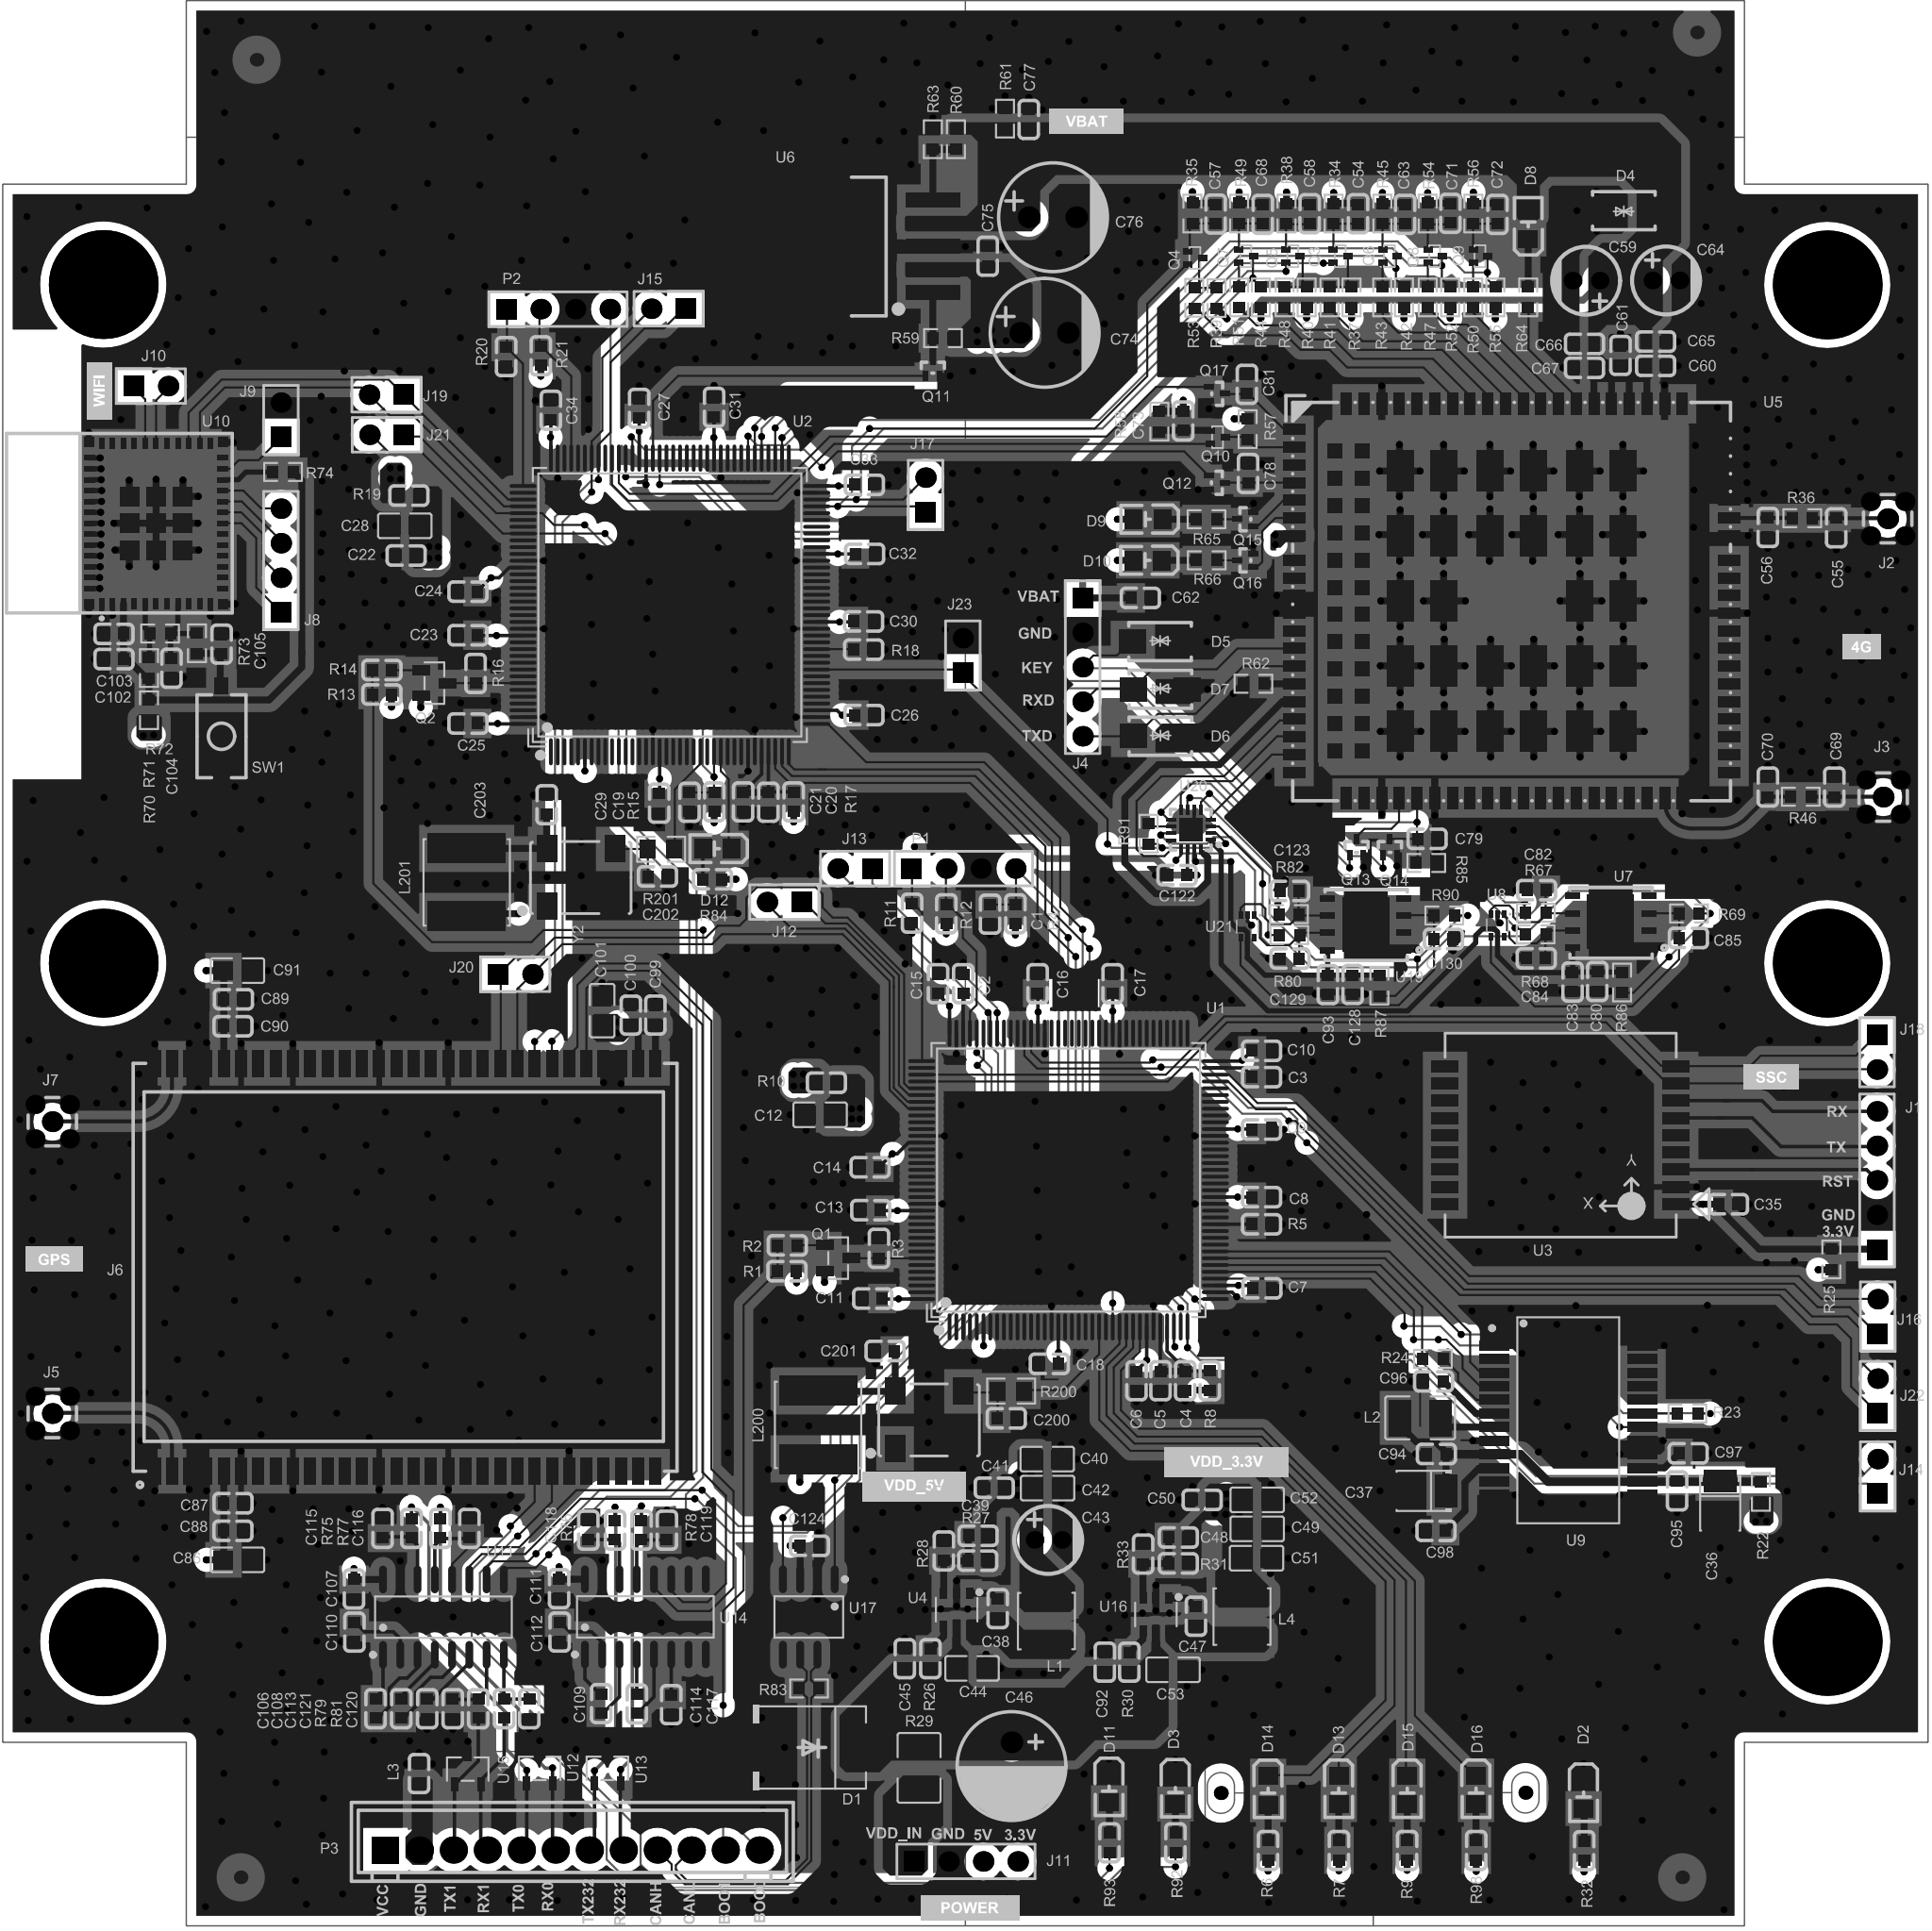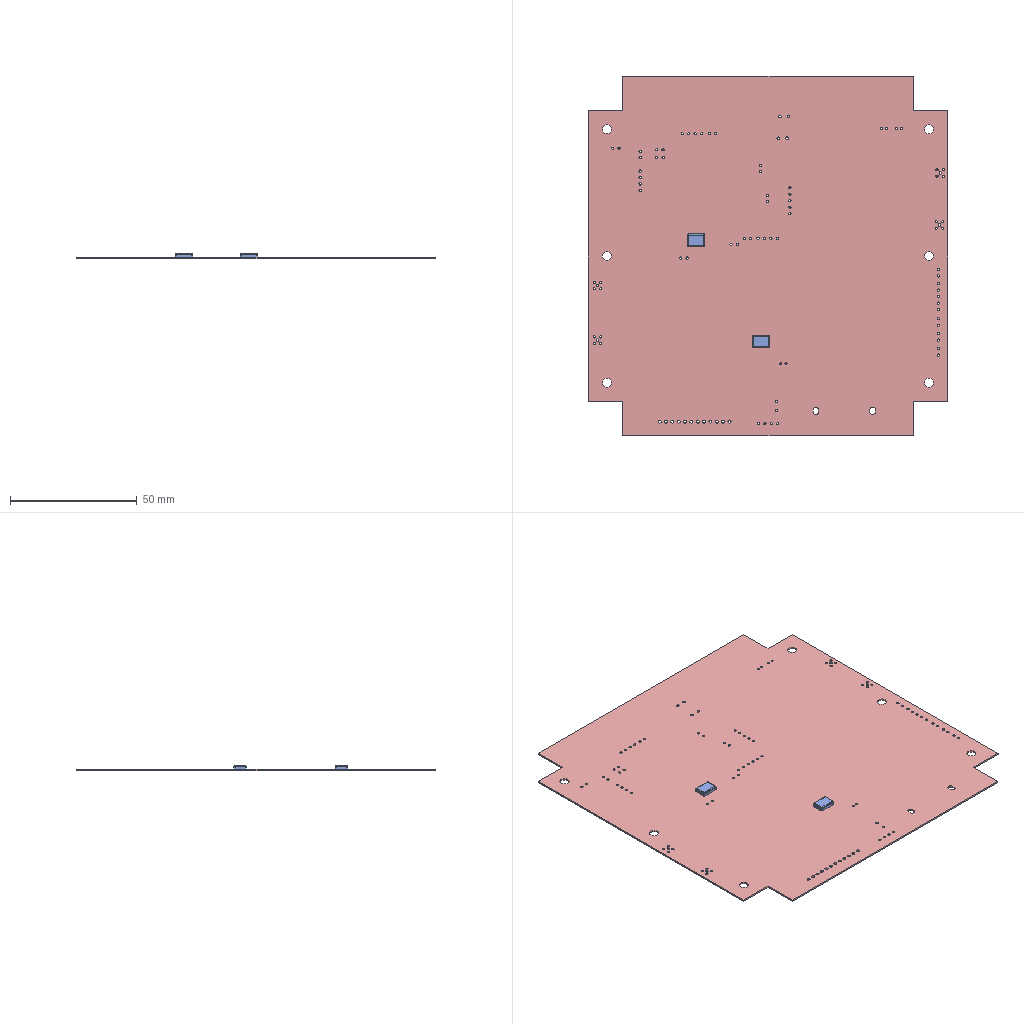Circuit board layout | Altium Designer | box 141.6 x 141.6 x 2.1 mm
Layer stack:
# Altium Designer layer stack of  (unit mm; dielectric type: 0 none, 1 core, 2 prepreg, 3 surface material)
index,name,kind,layer,copper_thickness_mm,dielectric_type,dielectric_thickness_mm,dielectric_material,dielectric_constant
0,Top Paste,other,,,,,,
1,Top Overlay,other,,,,,,
2,Top Solder,dielectric,,,3,0.0102,Solder Resist,3.5
3,Top,copper,Top,0.0356,,,,
4,Dielectric1,dielectric,,,2,0.0711,PP-006,4.1
5,GND02,copper,GND02,0.035,,,,
6,Dielectric5,dielectric,,,0,0.32,FR-4,4.8
7,PWR03,copper,PWR03,0.035,,,,
8,Dielectric6,dielectric,,,2,0.0711,PP-006,4.1
9,Bottom,copper,Bottom,0.0356,,,,
10,Bottom Solder,dielectric,,,3,0.0102,Solder Resist,3.5
11,Bottom Overlay,other,,,,,,
12,Bottom Paste,other,,,,,,
# drill layer pairs: low layer,high layer
drill_pair,Top,Bottom
Part placement:
Designator,Comment,Layer,Footprint,Center-X(mm),Center-Y(mm),Rotation
J11,Single-row straight pin header,TopLayer,HDR1X4,234.391,4.724,360
R85,10K,TopLayer,R0603,268.25,78.159,360
R84,NA,TopLayer,0603,215.74,76.965,180
J23,Boot Option-2.54-single-row pin header,TopLayer,HDR_1X2_254,234.163,93.421,90
J22,Boot Option-2.54-single-row pin header,TopLayer,HDR_1X2_254,301.447,38.964,90
J21,Boot Option-2.54-single-row pin header,TopLayer,HDR_1X2_254,191.795,109.652,180
J20,Boot Option-2.54-single-row pin header,TopLayer,HDR_1X2_254,201.244,69.977,360
J19,Boot Option-2.54-single-row pin header,TopLayer,HDR_1X2_254,191.77,112.598,180
J18,Boot Option-2.54-single-row pin header,TopLayer,HDR_1X2_254,301.396,64.237,270
J17,Boot Option-2.54-single-row pin header,TopLayer,HDR_1X2_254,231.419,105.232,90
J16,Boot Option-2.54-single-row pin header,TopLayer,HDR_1X2_254,301.447,44.806,90
J15,Boot Option-2.54-single-row pin header,TopLayer,HDR_1X2_254,212.522,118.923,180
J14,Boot Option-2.54-single-row pin header,TopLayer,HDR_1X2_254,301.447,33.045,90
J13,Boot Option-2.54-single-row pin header,TopLayer,HDR_1X2_254,226.238,77.749,180
D12,RED,TopLayer,LED_0805,216.089,79.209,360
C96,470nF/50V,TopLayer,0603,268.775,40.033,180
U21,ESDA6V8V6-6,TopLayer,SOT-563,255.092,73.482,90
U16,SY8113B,TopLayer,TSOT-23-6_L2.9-W1.6-P0.95-LS2.8-BR,248.361,22.885,90
U4,SY8113B,TopLayer,TSOT-23-6_L2.9-W1.6-P0.95-LS2.8-BR,233.705,23.241,90
R90,22R,TopLayer,R0603,269.571,74.297,180
R82,22R,TopLayer,R0603,258.149,74.397,360
R80,22R,TopLayer,R0603,258.174,72.859,360
R33,22.1K,TopLayer,0603,247.419,27.323,270
R32,1K,TopLayer,0603,279.854,5.504,270
R31,100K,TopLayer,0603,250.02,26.642,360
R30,100K,TopLayer,0603,246.403,19.372,270
R29,12V/2A,TopLayer,1210,230.944,11.607,270
R28,10K,TopLayer,0603,232.763,27.551,270
R27,75K 1%,TopLayer,0603,235.262,26.845,360
R26,100K,TopLayer,0603,231.772,19.627,270
R25,0R,TopLayer,R0603,298.04,48.997,90
R24,0R,TopLayer,R0603,268.733,41.685,360
R23,0R,TopLayer,R0603,287.451,37.665,180
R22,0R,TopLayer,R0603,292.859,31.903,90
L1,2.2uH/2A,TopLayer,IND-SMD_L4.0-W4.0,240.309,22.403,90
D11,RED,TopLayer,LED_0805,244.921,10.095,90
D3,RED,TopLayer,LED_0805,249.798,9.994,90
D2,RED,TopLayer,LED_0805,279.82,9.663,90
D1,SMCJ18A,TopLayer,SMC_L6.9-W5.9-LS7.9-RD,223.063,13.106,360
C123,33pF/50V,TopLayer,C0603,258.188,76.104,180
C122,100nF/50V,TopLayer,C0603,249.918,77.264,360
C53,10uF/25V,TopLayer,C0805,249.622,18.821,180
C52,22uF/10V,TopLayer,C0805,255.812,31.318,360
C51,22uF/10V,TopLayer,C0805,255.761,27.026,360
C50,100nF/50V,TopLayer,0603,251.757,31.321,180
C49,22uF/10V,TopLayer,C0805,255.812,29.185,360
C48,100pF/50V,TopLayer,0603,250.005,28.552,180
C47,100nF/50V,TopLayer,0603,251.31,22.766,90
C46,470uF/25V,TopLayer,CAP-TH_BD8.0-P3.50-D1.0-FD,237.744,11.739,270
C45,100nF/50V,TopLayer,0603,229.893,19.627,270
C44,10uF/25V,TopLayer,C0805,234.84,18.923,180
C43,100uF/10V,TopLayer,CAP-TH_BD5.0-P2.00-D0.8-FD,240.436,28.372,360
C42,22uF/10V,TopLayer,C0805,240.394,32.182,360
C41,100nF/50V,TopLayer,0603,236.466,32.21,180
C40,22uF/10V,TopLayer,C0805,240.369,34.315,360
C39,100pF/50V,TopLayer,0603,235.273,28.679,180
C38,100nF/50V,TopLayer,0603,236.731,23.325,90
C37,47uF/10V,TopLayer,CAP-SMD_L3.5-W2.8,267.894,31.979,0
C36,47uF/10V,TopLayer,CAP-SMD_L3.5-W2.8,289.865,30.886,90
SW1,TS-1101-B-W,TopLayer,SMD,179.64,87.479,90
Y2,8MHZ 3.3V 20PPM,TopLayer,XTAL_5.7X7.0-SM_-_duplicate,206.061,77.089,360
Y1,8MHZ 3.3V 20PPM,TopLayer,XTAL_5.7X7.0-SM_-_duplicate,231.678,37.195,360
R201,10R 1%,TopLayer,R0805,211.971,79.169,180
R200,10R 1%,TopLayer,R0805,237.715,39.319,180
L201,1uH 10%,TopLayer,SMD_L6.0-W6.0,197.672,76.73,270
L200,1uH 10%,TopLayer,SMD_L6.0-W6.0,223.516,36.831,270
C203,100nF/50V,TopLayer,C0603,203.557,82.452,90
C202,15pF/50V,TopLayer,C0603,211.695,77.172,180
C201,100nF/50V,TopLayer,C0603,228.436,42.27,180
C200,15pF/50V,TopLayer,C0603,237.351,37.317,180
U20,FSA2567MPX,TopLayer,TQFN-16_L3.0-W3.0-P0.50-BL-EP1.7,250.93,80.595,90
U19,China Telecom eSIM,TopLayer,DFN-8_L6.0-W5.0-P1.27-BL-EP-A,263.8,73.661,90
U17,TJA1050T/CM,118,TopLayer,SOIC-8,222.834,22.704,180
U15,PESD15VL2BT,TopLayer,SOT-23,197.749,11.515,270
U14,SP3232EEN,TopLayer,SOP16-6_6,210.812,22.711,360
U13,PESD15VL2BT,TopLayer,SOT-23,208.02,11.572,270
U12,PESD15VL2BT,TopLayer,SOT-23,203.037,11.566,270
U11,SP3232EEN,TopLayer,SOP16-6_6,195.961,22.691,360
U9,SCC2130,TopLayer,SCC2130D,278.689,37.171,270
U8,ESDA6V8V6-6,TopLayer,SOT-563,273.482,73.558,90
U7,China Mobile eSIM,TopLayer,DFN-8_L6.0-W5.0-P1.27-BL-EP-A,281.814,73.825,90
U6,MIC29302WU,TopLayer,TO-263-5,226.621,123.499,180
U5,EC25/EC21_U17,TopLayer,EC20,274.523,97.434,270
U2,STM32F103ZET6,TopLayer,LQFP144-20x20mm,212.613,97.138,360
U1,STM32F407ZET6,TopLayer,LQFP144-20x20mm,241.935,54.839,360
R98,NA,TopLayer,0603,271.922,5.538,90
R93,NA,TopLayer,0603,244.949,6.1,90
R92,NA,TopLayer,0603,249.8,6.1,90
R91,NM,TopLayer,R0603,247.825,80.315,90
R83,120R,TopLayer,R0603,222.852,17.443,180
R81,4.7Ω,±1%,TopLayer,0603,200.427,15.961,90
R79,4.7Ω,±1%,TopLayer,0603,198.524,15.961,90
R78,4.7Ω,±1%,TopLayer,0603,210.525,29.08,270
R77,4.7Ω,±1%,TopLayer,0603,195.736,29.207,270
R76,4.7Ω,±1%,TopLayer,0603,208.582,29.08,270
R75,4.7Ω,±1%,TopLayer,0603,193.609,29.207,270
R74,10K,TopLayer,R0603,184.166,106.919,180
R73,0R,TopLayer,R0603,177.835,94.32,270
R72,10K,TopLayer,R0603,175.121,95.036,360
R71,10K,TopLayer,R0603,174.306,92.495,270
R70,0R,TopLayer,R0603,174.306,89.396,90
R69,22R,TopLayer,R0603,287.57,74.447,180
R68,22R,TopLayer,R0603,276.284,72.909,360
R67,22R,TopLayer,R0603,276.31,74.496,360
R66,4.7K,TopLayer,R0603,252.101,100.418,360
R65,4.7K,TopLayer,R0603,252.085,103.441,360
R64,4.7K,TopLayer,R0603,275.744,119.756,270
R63,47K,TopLayer,R0603,231.957,131.39,270
R62,NM,TopLayer,R0603,255.534,91.34,360
R61,330R,TopLayer,R0603,237.263,132.906,270
R60,100K,TopLayer,R0603,233.653,131.389,90
R59,47K,TopLayer,R0603,232.702,116.763,360
R58,4.7K,TopLayer,R0603,248.616,110.628,270
R57,4.7K,TopLayer,R0603,255.109,110.073,270
R56,4.7K,TopLayer,R0603,271.71,125.926,270
R55,10K,TopLayer,R0603,273.327,119.756,270
R54,4.7K,TopLayer,R0603,268.353,125.926,270
R53,0R,TopLayer,R0603,251.186,119.73,270
R52,10K,TopLayer,R0603,270.004,119.756,270
R51,0R,TopLayer,R0603,254.483,119.756,270
R50,0R,TopLayer,R0603,271.704,119.756,270
R49,4.7K,TopLayer,R0603,254.482,125.926,270
R48,0R,TopLayer,R0603,257.83,119.756,270
R47,0R,TopLayer,R0603,268.356,119.756,270
R46,0R,TopLayer,R0603,295.789,83.034,360
R45,4.7K,TopLayer,R0603,265.021,125.926,270
R44,10K,TopLayer,R0603,256.085,119.756,270
R43,0R,TopLayer,R0603,265.008,119.756,270
R42,10K,TopLayer,R0603,266.606,119.756,270
R41,0R,TopLayer,R0603,261.127,119.756,270
R40,10K,TopLayer,R0603,259.447,119.756,90
R39,10K,TopLayer,R0603,252.826,119.705,90
R38,4.7K,TopLayer,R0603,257.97,125.926,90
R37,10K,TopLayer,R0603,262.75,119.756,90
R36,0R,TopLayer,R0603,295.901,103.516,360
R35,4.7K,TopLayer,R0603,251.048,125.926,90
R34,4.7K,TopLayer,R0603,261.435,125.926,90
R21,10K,TopLayer,0603,203.12,115.457,270
R20,10K,TopLayer,0603,200.571,115.396,270
R19,0R,TopLayer,0603,193.429,105.179,360
R18,10K,TopLayer,0603,226.859,93.856,180
R17,120R@100MHz,TopLayer,0603,221.719,82.659,90
R16,10K,TopLayer,0603,198.321,92.093,270
R15,10K,TopLayer,0603,215.872,82.644,270
R14,10K,TopLayer,0603,191.432,92.353,180
R13,10K,TopLayer,0603,191.441,90.548,360
R12,10K,TopLayer,0603,232.941,74.414,270
R11,10K,TopLayer,0603,230.426,74.459,270
R10,0R,TopLayer,0603,224.137,61.999,360
R9,NA,TopLayer,0603,266.84,5.538,90
R8,120R@100MHz,TopLayer,0603,252.326,40.089,90
R7,NA,TopLayer,0603,261.825,5.538,90
R6,NA,TopLayer,0603,256.611,5.538,90
R5,10K,TopLayer,0603,256.126,51.59,180
R4,10K,TopLayer,0603,238.025,74.414,270
R3,10K,TopLayer,0603,227.988,49.808,270
R2,10K,TopLayer,0603,221.245,50.038,180
R1,10K,TopLayer,0603,221.235,48.13,360
Q17,DTC043ZEBTL,TopLayer,SOT-416_L1_6-W0_8-P1_00-LS1_6-BR,252.871,112.664,180
Q16,DTC043ZEBTL,TopLayer,SOT-416_L1_6-W0_8-P1_00-LS1_6-BR,254.943,100.418,360
Q15,DTC043ZEBTL,TopLayer,SOT-416_L1_6-W0_8-P1_00-LS1_6-BR,254.943,103.441,360
Q14,DTC043ZEBTL,TopLayer,SOT-416_L1_6-W0_8-P1_00-LS1_6-BR,265.574,79.333,270
Q13,DTC043ZEBTL,TopLayer,SOT-416_L1_6-W0_8-P1_00-LS1_6-BR,263.117,79.333,270
Q12,DTC043ZEBTL,TopLayer,SOT-416_L1_6-W0_8-P1_00-LS1_6-BR,252.846,106.122,180
Q11,DTC043ZEBTL,TopLayer,SOT-416_L1_6-W0_8-P1_00-LS1_6-BR,231.954,114.588,270
Q10,2SC4617TLQ,TopLayer,EMT3,252.92,109.481,180
Q9,2SC4617TLQ,TopLayer,EMT3,272.218,122.787,180
Q8,2SC4617TLQ,TopLayer,EMT3,268.887,122.787,180
Q7,2SC4617TLQ,TopLayer,EMT3,254.998,122.787,180
Q6,2SC4617TLQ,TopLayer,EMT3,265.555,122.787,180
Q5,2SC4617TLQ,TopLayer,EMT3,258.456,122.787,180
Q4,2SC4617TLQ,TopLayer,EMT3,251.252,122.66,180
Q3,2SC4617TLQ,TopLayer,EMT3,261.943,122.787,180
Q2,8550,TopLayer,SOT-23-SS8550,195.296,91.387,180
Q1,8550,TopLayer,SOT-23-SS8550,224.993,49.098,180
P3,Through-hole pad, 2mm pitch,TopLayer,XH-12A,205.445,5.564,360
P2,Single-row straight pin header,TopLayer,HDR1X4,204.39,118.894,360
P1,Single-row straight pin header,TopLayer,HDR1X4,234.213,77.749,360
L4,2.2uH/2A,TopLayer,IND-SMD_L4.0-W4.0,254.693,22.734,90
L3,120Ω ±25% @100MHz,TopLayer,0603,194.173,11.194,90
L2,47uH±20%,TopLayer,1210,267.795,37.349,360
J10,Boot Option-2.54-single-row pin header,TopLayer,HDR_1X2_254,174.447,113.233,360
J9,Boot Option-2.54-single-row pin header,TopLayer,HDR_1X2_254,184.008,110.745,90
J8,JTAG-4p-2.54-single-row pin header,TopLayer,HDR_1X4_254,184.008,100.407,90
J7,MMCX-KE RF connector,TopLayer,MMCX-KE,167.197,59.132,180
J6,UM482/K823,TopLayer,UM482_K823,193.142,48.422,90
J5,MMCX-KE RF connector,TopLayer,MMCX-KE,167.197,37.668,270
J4,HEADER 5,TopLayer,2.54mm_paizhen_5pin,242.975,92.559,360
J3,MMCX-KE RF connector,TopLayer,MMCX-KE,301.853,83.005,360
J2,MMCX-KE RF connector,TopLayer,MMCX-KE,302.184,103.48,270
D16,RED,TopLayer,LED_0805,271.908,9.955,90
D15,RED,TopLayer,LED_0805,266.851,9.955,90
D14,RED,TopLayer,LED_0805,256.616,9.948,90
D13,RED,TopLayer,LED_0805,261.811,9.955,90
D10,GREEN,TopLayer,LED0805,247.763,100.418,360
D9,GREEN,TopLayer,LED0805,247.788,103.44,360
D8,GREEN,TopLayer,LED0805,275.744,125.103,270
D7,SMAJ6.8CA,TopLayer,SMA,248.693,90.934,180
D6,SMAJ6.8CA,TopLayer,SMA,248.693,87.48,180
D5,SMAJ6.8CA,TopLayer,SMA,248.667,94.439,180
D4,SMAJ6.8CA,TopLayer,SMA,282.777,126.135,360
C130,33pF/50V,TopLayer,C0603,269.519,72.567,360
C129,33pF/50V,TopLayer,C0603,258.217,71.134,180
C128,33pF/50V,TopLayer,C0603,262.828,69.216,270
C124,100nF/50V,TopLayer,C0603,222.874,27.945,180
C121,15pF/50V,TopLayer,0603,196.642,15.946,270
C120,15pF/50V,TopLayer,0603,202.273,15.946,270
C119,15pF/50V,TopLayer,0603,212.392,29.08,270
C118,15pF/50V,TopLayer,0603,206.613,29.08,270
C117,100nF/50V,TopLayer,0603,212.713,16.251,270
C116,15pF/50V,TopLayer,0603,197.863,29.207,270
C115,15pF/50V,TopLayer,0603,191.482,29.207,270
C114,100nF/50V,TopLayer,0603,210.189,16.317,90
C113,100nF/50V,TopLayer,0603,194.766,15.946,270
C112,100nF/50V,TopLayer,0603,204.505,21.587,270
C111,100nF/50V,TopLayer,0603,204.468,24.777,270
C110,100nF/50V,TopLayer,0603,189.412,21.585,270
C109,100nF/50V,TopLayer,0603,207.568,16.343,90
C108,100nF/50V,TopLayer,0603,192.861,15.961,90
C107,100nF/50V,TopLayer,0603,189.38,24.757,270
C106,100nF/50V,TopLayer,0603,190.97,15.961,90
C105,100nF/50V,TopLayer,C0603,179.646,94.266,90
C104,100nF/50V,TopLayer,C0603,175.959,92.49,90
C103,100nF/50V,TopLayer,C0603,171.738,95.008,360
C102,100nF/50V,TopLayer,C0603,171.738,93.154,360
C101,10uF/25V,TopLayer,C0805,207.633,67.298,270
C100,100nF/50V,TopLayer,0603,209.739,66.959,270
C99,100pF/50V,TopLayer,0603,211.542,66.966,270
C98,1uF/25V,TopLayer,0603,268.953,29.045,180
C97,1uF/25V,TopLayer,0603,287.517,34.74,360
C95,100nF/50V,TopLayer,0603,286.692,31.971,270
C94,1uF/25V,TopLayer,0603,268.983,34.696,180
C93,100nF/50V,TopLayer,C0603,261.008,69.207,270
C92,100nF/50V,TopLayer,0603,244.602,19.374,270
C91,10uF/25V,TopLayer,C0805,180.811,70.243,180
C90,100nF/50V,TopLayer,0603,180.475,66.156,180
C89,100pF/50V,TopLayer,0603,180.51,68.137,180
C88,100pF/50V,TopLayer,0603,180.485,29.04,360
C87,100nF/50V,TopLayer,0603,180.492,31.069,360
C86,10uF/25V,TopLayer,C0805,180.815,26.906,180
C85,33pF/50V,TopLayer,C0603,287.536,72.641,360
C84,33pF/50V,TopLayer,C0603,276.327,71.146,180
C83,33pF/50V,TopLayer,C0603,279.005,69.393,270
C82,33pF/50V,TopLayer,C0603,276.353,76.161,180
C81,10nF,TopLayer,C0603,255.054,113.37,90
C80,100nF/50V,TopLayer,C0603,280.82,69.436,270
C79,10nF,TopLayer,C0603,268.315,79.932,360
C78,10nF,TopLayer,C0603,255.142,106.817,90
C77,100nF/50V,TopLayer,C0603,239.015,132.852,90
C76,470uF/25V,TopLayer,RB8*11_5,240.756,125.654,360
C75,100nF/50V,TopLayer,C0603,235.993,122.795,90
C74,470uF/25V,TopLayer,RB8*11_5,240.138,117.153,360
C73,1nF/50V,TopLayer,C0603,250.372,110.677,90
C72,1nF/50V,TopLayer,C0603,273.482,125.87,90
C71,1nF/50V,TopLayer,C0603,270.023,125.946,90
C70,NM,TopLayer,C0603,293.367,83.736,270
C69,NM,TopLayer,C0603,298.252,83.734,270
C68,1nF/50V,TopLayer,C0603,256.224,125.87,90
C67,12pF/50V,TopLayer,C0603,279.876,114.58,180
C66,33pF/50V,TopLayer,C0603,279.876,116.339,180
C65,100nF/50V,TopLayer,C0603,285.122,116.503,360
C64,100uF/10V,TopLayer,RB5*7,285.884,121.001,360
C63,1nF/50V,TopLayer,C0603,266.691,125.87,90
C62,12pF/50V,TopLayer,C0603,247.225,97.654,360
C61,33pF/50V,TopLayer,C0603,282.533,115.501,90
C60,100nF/50V,TopLayer,C0603,285.122,114.723,360
C59,100uF/10V,TopLayer,RB5*7,280.003,120.987,180
C58,1nF/50V,TopLayer,C0603,259.666,125.905,270
C57,1nF/50V,TopLayer,C0603,252.749,125.88,270
C56,NM,TopLayer,C0603,293.369,102.844,90
C55,NM,TopLayer,C0603,298.401,102.819,90
C54,1nF/50V,TopLayer,C0603,263.227,125.905,270
C34,100nF/50V,TopLayer,C0603,203.862,111.464,90
C33,100nF/50V,TopLayer,C0603,226.929,105.969,360
C32,100nF/50V,TopLayer,C0603,226.947,100.889,360
C31,100nF/50V,TopLayer,C0603,215.869,111.682,90
C30,100nF/50V,TopLayer,C0603,226.871,95.922,360
C29,100nF/50V,TopLayer,C0603,211.828,82.552,270
C28,4.7uF/10V,TopLayer,C0805,193.119,102.958,180
C27,100nF/50V,TopLayer,C0603,210.358,111.606,90
C26,100nF/50V,TopLayer,C0603,226.896,89.037,360
C25,100nF/50V,TopLayer,C0603,197.757,88.417,180
C24,100nF/50V,TopLayer,C0603,197.757,98.116,180
C23,100nF/50V,TopLayer,C0603,197.757,94.912,180
C22,100nF/50V,TopLayer,C0603,193.21,100.776,180
C21,10uF/10V,TopLayer,C0603,217.998,82.644,270
C20,10uF/10V,TopLayer,C0603,219.856,82.618,270
C19,100nF/50V,TopLayer,0603,214.062,82.634,90
C18,100nF/50V,TopLayer,C0603,240.514,41.326,180
C17,100nF/50V,TopLayer,C0603,245.18,69.289,90
C16,100nF/50V,TopLayer,C0603,239.662,69.289,90
C15,100nF/50V,TopLayer,C0603,232.341,69.289,90
C14,100nF/50V,TopLayer,C0603,227.332,55.78,180
C13,100nF/50V,TopLayer,C0603,227.383,52.624,180
C12,4.7uF/10V,TopLayer,C0805,223.664,59.639,180
C11,100nF/50V,TopLayer,C0603,227.525,46.126,180
C10,100nF/50V,TopLayer,C0603,256.141,64.342,360
C9,100nF/50V,TopLayer,C0603,256.141,58.555,360
C8,100nF/50V,TopLayer,C0603,256.141,53.58,360
C7,100nF/50V,TopLayer,C0603,256.167,46.878,360
C6,100nF/50V,TopLayer,C0603,246.932,40.073,270
C5,10uF/10V,TopLayer,C0603,248.701,40.073,270
C4,10uF/10V,TopLayer,C0603,250.511,40.073,270
C3,2.2uF/25V,TopLayer,C0603,256.141,62.408,360
C2,2.2uF/25V,TopLayer,C0603,234.191,69.289,90
C1,100nF/50V,TopLayer,0603,236.169,74.404,90
J1,HEADER 5,TopLayer,2.54mm_paizhen_5pin,301.396,54.813,180
U3,FSS-IMU614E-P1,TopLayer,FSS-IMU614E-P1,278.13,58.141,180
C35,100nF/50V,TopLayer,0603,290.482,53.058,360
U10,ESP32-C3-MINI-1U,TopLayer,WIFIM-SMD_ESP32-C3-MINI-1,174.828,103.149,90
J12,Boot Option-2.54-single-row pin header,TopLayer,HDR_1X2_254,221.031,75.286,180
R86,10K,TopLayer,R0603,282.648,69.368,90
R87,10K,TopLayer,R0603,264.798,69.138,270
Pad and via stacks:
# Altium Designer via and pad stacks of  (unit mm). Each distinct definition once, with the count of objects using it.
# via: kind,start_layer,end_layer,hole_mm,diameter_mm,mode(0 simple;1 top-mid-bottom;2 full stack),diameter_per_layer,count,example_net
# pad: kind,layer,hole_mm,hole_type(0 round;1 square;2 slot),plating,top_size,top_shape(1 round;2 rect;3 octagon;9 rounded rect),mid_size,bottom_size,mode,footprint,size_per_layer,count,example
pad,Top,0,0,plated,0.8065x0.864,2,0.8065x0.864,0.8065x0.864,0,R0603,,106,R85.2
pad,Top,0,0,plated,1.3x1.399,2,1.3x1.399,1.3x1.399,0,LED_0805,,16,D12.2
pad,Top,0,0,plated,0.8x0.9,2,0.8x0.9,0.8x0.9,0,0603,,154,R84.2
pad,Top,0,0,plated,0.8x0.9,2,0.8x0.9,0.8x0.9,0,C0603,,146,C123.1
pad,Top,0,0,plated,0.3x0.5,2,0.3x0.5,0.3x0.5,0,SOT-563,,12,U21.6
pad,Top,0,0,plated,0.45x1.1,2,0.45x1.1,0.45x1.1,0,DFN-8_L6.0-W5.0-P1.27-BL-EP-A,,16,U19.1
pad,Top,0,0,plated,4x3.4,2,4x3.4,4x3.4,0,DFN-8_L6.0-W5.0-P1.27-BL-EP-A,,2,U19.9
pad,Top,0,0,plated,1.6x3.5,2,1.6x3.5,1.6x3.5,0,IND-SMD_L4.0-W4.0,,4,L1.2
pad,Top,0,0,plated,0.8x0.532,2,0.8x0.532,0.8x0.532,0,TSOT-23-6_L2.9-W1.6-P0.95-LS2.8-BR,,12,U4.6
pad,Top,0,0,plated,1.41x1.35,2,1.41x1.35,1.41x1.35,0,C0805,,24,C42.2
pad,Top,0,0,plated,1.635x2.7,2,1.635x2.7,1.635x2.7,0,1210,,4,R29.1
pad,Top,0,0,plated,2.7x3.3,2,2.7x3.3,2.7x3.3,0,SMC_L6.9-W5.9-LS7.9-RD,,2,D1.2
pad,Top,0,0,plated,1.607x2.376,2,1.607x2.376,1.607x2.376,0,CAP-SMD_L3.5-W2.8,,4,C36.1
pad,Top,0,0,plated,1.7x1.7,2,1.7x1.7,1.7x1.7,0,TQFN-16_L3.0-W3.0-P0.50-BL-EP1.7,,1,U20.17
pad,Top,0,0,plated,0.75x0.25,2,0.75x0.25,0.75x0.25,0,TQFN-16_L3.0-W3.0-P0.50-BL-EP1.7,,8,U20.16
pad,Top,0,0,plated,0.25x0.75,2,0.25x0.75,0.25x0.75,0,TQFN-16_L3.0-W3.0-P0.50-BL-EP1.7,,8,U20.12
pad,Top,0,0,plated,1.25x0.7,2,1.25x0.7,1.25x0.7,0,SOT-23-SS8550,,6,Q2.1
pad,Top,0,0,plated,0.28x2,1,0.28x2,0.28x2,0,LQFP144-20x20mm,,144,U2.1
pad,Top,0,0,plated,2x0.28,1,2x0.28,2x0.28,0,LQFP144-20x20mm,,144,U2.37
pad,Top,0,0,plated,2.2x5.72,2,2.2x5.72,2.2x5.72,0,SMD_L6.0-W6.0,,4,L201.2
pad,Top,0,0,plated,1.133x1.377,2,1.133x1.377,1.133x1.377,0,R0805,,4,R201.1
pad,Top,0,0,plated,1.5x2,2,1.5x2,1.5x2,0,XTAL 5.7X7.0-SM - duplicate,,8,Y2.4
pad,Top,0,0,plated,1.2x1,2,1.2x1,1.2x1,0,SMD,,2,SW1.1
pad,Top,0,0,plated,0.574x2.038,1,0.574x2.038,0.574x2.038,0,SOP16-6_6,,32,U14.1
pad,Top,0,0,plated,2.01x0.85,2,2.01x0.85,2.01x0.85,0,UM482_K823,,60,J6.60
pad,Top,0,0,plated,10.66x8.89,2,10.66x8.89,10.66x8.89,0,TO-263-5,,1,U6.6
pad,Top,0,0,plated,4x1.069,2,4x1.069,4x1.069,0,TO-263-5,,5,U6.5
pad,Top,0,0,plated,0.4603x0.65,2,0.4603x0.65,0.4603x0.65,0,EMT3,,8,Q10.3
pad,Top,0,0,plated,0.46x0.6502,2,0.46x0.6502,0.46x0.6502,0,EMT3,,16,Q10.1
pad,Top,0,0,plated,0.7x2.2,2,0.7x2.2,0.7x2.2,0,SCC2130D,,24,U9.24
pad,Top,0,0,plated,0.4x0.7,2,0.4x0.7,0.4x0.7,0,SOT-416_L1_6-W0_8-P1_00-LS1_6-BR,,21,Q11.3
pad,Top,0,0,plated,1.1x1.1,2,1.1x1.1,1.1x1.1,0,EC20,,24,U5.140
pad,Top,0,0,plated,1.625x0.8,2,1.625x0.8,1.625x0.8,0,EC20,,76,U5.1
pad,Top,0,0,plated,3x2,2,3x2,3x2,0,EC20,,28,U5.85
pad,Top,0,0,plated,0.8x1.625,2,0.8x1.625,0.8x1.625,0,EC20,,4,U5.141
pad,Top,0,0,plated,2x1.8,2,2x1.8,2x1.8,0,SMA,,8,D4.1
pad,Top,0,0,plated,1.038x0.532,2,1.038x0.532,1.038x0.532,0,SOT-23,,9,U13.3
pad,Top,0,0,plated,1.3x1.399,2,1.3x1.399,1.3x1.399,0,LED0805,,6,D10.2
pad,Top,0,0,plated,2x0.85,2,2x0.85,2x0.85,0,FSS-IMU614E-P1,,18,U3.1
pad,Top,0,0,unplated,1x1,1,1x1,1x1,0,,,4,MARK
pad,Top,0,0,plated,0.588x2.045,1,0.588x2.045,0.588x2.045,0,SOIC-8,,8,U17.1
pad,Top,0,0,plated,1.45x1.45,2,1.45x1.45,1.45x1.45,0,WIFIM-SMD_ESP32-C3-MINI-1,,9,U10.49
pad,Top,0,0,plated,0.4x0.8,2,0.4x0.8,0.4x0.8,0,WIFIM-SMD_ESP32-C3-MINI-1,,48,U10.1
pad,Top,0,0,plated,0.7x0.7,2,0.7x0.7,0.7x0.7,0,WIFIM-SMD_ESP32-C3-MINI-1,,4,U10.50
pad,Multi-Layer,0.9,0,plated,1.5x1.5,1,1.5x1.5,1.5x1.5,0,HDR1X4,,9,J11.4
pad,Multi-Layer,0.9,0,plated,1.5x1.5,2,1.5x1.5,1.5x1.5,0,HDR1X4,,3,J11.1
pad,Multi-Layer,0.9144,0,plated,1.499x1.499,2,1.499x1.499,1.499x1.499,0,HDR_1X2_254,,14,J23.1
pad,Multi-Layer,0.9144,0,plated,1.499x1.499,1,1.499x1.499,1.499x1.499,0,HDR_1X2_254,,14,J23.2
pad,Multi-Layer,0.9144,0,plated,1.499x1.499,1,1.499x1.499,1.499x1.499,0,HDR_1X4_254,,3,J8.4
pad,Multi-Layer,0.9144,0,plated,1.499x1.499,2,1.499x1.499,1.499x1.499,0,HDR_1X4_254,,1,J8.1
pad,Multi-Layer,0.8,0,plated,1.3x1.3,1,1.3x1.3,1.3x1.3,0,CAP-TH_BD5.0-P2.00-D0.8-FD,,2,C43.1
pad,Multi-Layer,1,0,plated,1.6x1.6,1,1.6x1.6,1.6x1.6,0,CAP-TH_BD8.0-P3.50-D1.0-FD,,2,C46.1
pad,Multi-Layer,2.1,2,unplated,1.016x1.016,1,1.016x1.016,1.016x1.016,0,,,2,1
pad,Multi-Layer,3.6,0,plated,8x8,1,8x8,8x8,0,,,6,0
pad,Multi-Layer,1,0,plated,1.524x1.524,1,1.524x1.524,1.524x1.524,0,MMCX-KE,,4,J7.1
pad,Multi-Layer,0.9,0,plated,1.4x1.4,1,1.4x1.4,1.4x1.4,0,MMCX-KE,,16,J7.2
pad,Multi-Layer,1,0,plated,1.6x1.6,1,1.6x1.6,1.6x1.6,0,RB8*11_5,,4,C76.1
pad,Multi-Layer,0.9144,0,plated,1.499x1.499,1,1.499x1.499,1.499x1.499,0,2.54mm_paizhen_5pin,,8,J4.5
pad,Multi-Layer,0.9144,0,plated,1.499x1.499,2,1.499x1.499,1.499x1.499,0,2.54mm_paizhen_5pin,,2,J4.1
pad,Multi-Layer,0.8,0,plated,1.3x1.3,1,1.3x1.3,1.3x1.3,0,RB5*7,,4,C59.1
pad,Multi-Layer,1.2,0,plated,2x2,1,2x2,2x2,0,XH-12A,,11,P3.12
pad,Multi-Layer,1.2,0,plated,2x2,2,2x2,2x2,0,XH-12A,,1,P3.1
via,Top,Bottom,0.3048,0.508,0,,1701,VDD_3.3
Copper pours:
name,layer,net,type(0 solid;1 hatched;2 none)
BottomLayer-No Net,Top,VDD_3.3,0
BottomLayer-No Net,Top,VDD_5V,0
BottomLayer-No Net,Top,NetC47_1,0
BottomLayer-No Net,Top,NetC38_1,0
BottomLayer-No Net,Top,VDD_12V,0
BottomLayer-No Net,Top,VDD_IN,0
BottomLayer-No Net,Top,GND_IN,0
BottomLayer-No Net,Top,VDD_3.3,0
BottomLayer-No Net,Top,VDD_3.3,0
BottomLayer-No Net,Top,VDD_3.3,0
BottomLayer-No Net,Top,VDD_3.3,0
BottomLayer-No Net,Top,VDD_3.3,0
BottomLayer-No Net,Top,MCU1_VCC,0
BottomLayer-No Net,Top,MCU2_VCC,0
BottomLayer-No Net,Top,VDD_5V,0
BottomLayer-No Net,Top,VDD_EXT,0
BottomLayer-No Net,Top,VBAT,0
BottomLayer-No Net,Top,GND,0
BottomLayer-No Net,Bottom,GND,0
Design rules, without the lines most boards share:
# Altium Designer design rules of  (exported by Altium Designer, unit mm)
# columns: name | kind | enabled | priority | scope1 | scope2 | descriptor | typed fields (field=value)
SilkToSolderMaskClearance | 54 | enabled | 1 | IsPad | All | Silk To Solder Mask (Clearance=2mil) (IsPad),(All) |
HoleToHoleClearance | 52 | enabled | 1 | All | All | Hole To Hole Clearance (Gap=10mil) (All),(All) | gap=0.254
DiffPairsRouting | 51 | enabled | 1 | All | All | Differential Pairs Uncoupled Length using the Gap Constraints (Min=6mil) (Max=6mil) (Prefered=6mil)  and Width Constraints (Min=15mil) (Max=15mil) (Prefered=15mil) (All) |
SolderMaskExpansion | 13 | enabled | 1 | All | All | Solder Mask Expansion (Expansion =4mil) (All) | expansion=0.1016
RoutingVias | 11 | enabled | 1 | All | All | Routing Via (MinHoleWidth=12mil) (MaxHoleWidth=12mil) (PreferredHoleWidth=12mil) (MinWidth=20mil) (MaxWidth=20mil) (PreferedWidth=20mil) (All) | via_min_hole=0.3048 via_max_hole=0.3048 via_preferred_diameter=0.508 via_preferred_hole=0.3048
Width | 2 | enabled | 1 | All | All | Width Constraint (Min=6mil) (Max=60mil) (Preferred=6mil) (All) |
PolygonConnect | 20 | enabled | 1 | All | All | Polygon Connect Rule(Direct Connect )(Conductor Width=10mil) (Relief Angle=90 Angle) (Entries=4) (Air Gap Width=10mil) (All),(All) | connect_style(0=relief,1=direct,2=none)=1 relief_conductor_width=0.254 relief_entries=4
PlaneClearance | 12 | enabled | 1 | All | All | Power Plane Clearance (Clearance =10mil) (All) | clearance=0.254
PlaneConnect | 6 | enabled | 1 | All | All | Power Plane Connect Rule(Direct Connect )(Expansion=20mil) (Conductor Width=10mil) (Air Gap=10mil) (Entries=4) (All) | relief_conductor_width=0.254 relief_entries=4 relief_expansion=0.508
Clearance | 0 | enabled | 3 | All | All | Clearance Constraint (Gap=6mil) (All),(All) | gap=0.1524
Clearance_1 | 0 | enabled | 2 | INPOLYGON | All | Clearance Constraint (Gap=15mil) (INPOLYGON),(All) | gap=0.381
Clearance_2 | 0 | enabled | 1 | HASPAD('free-MARK') | All | Clearance Constraint (Gap=50mil) (HASPAD('free-MARK')),(All) | gap=1.27
Classes set for this board:
# Altium Designer classes of  (member kind: 0 net, 1 component, 2 from-to, 3 pad, 4 layer, 5 differential pair, 6 design channel, 7 polygon, 8 structure, 9 xSignal)
# columns: class name | member kind | superclass | members
06 4G_Comm | 1 | no | C54; C55; C56; C57; C58; C59; C60; C61; C62; C63; C64; C65; C66; C67; C68; C69; C70; C71; C72; C73; C74; C75; C76; C77; C78; C79; C80; C81; C82; C83; C84; C85; D4; D5; D6; D7; D8; D9; D10; J2; J3; J4; Q3; Q4; Q5; Q6; Q7; Q8; Q9; Q10; Q11; Q12; Q13; Q14; Q15; Q16; Q17; R34; R35; R36; R37; R38; R39; R40; R41; R42; R43; R44; R45; R46; R47; R48; R49; R50; R51; R52; R53; R54; R55; R56; R57; R58; R59; R60; R61; R62; R63; R64; R65; R66; R67; R68; R69; U5; U6; U7; U8; C93; C122; C123; C128; C129; C130; R80; R82; R90; R91; U19; U20; U21; J23; R85; R86; R87;
09 Power | 1 | no | L3; L4; C38; C39; C40; C41; C42; C43; C44; C45; C46; C47; C48; C49; C50; C51; C52; C53; C92; D1; D2; L1; R26; R27; R28; R29; R30; R31; R32; R33; U4; U16; J11;
08 Interface | 1 | no | C106; C107; C108; C109; C110; C111; C112; C113; C114; C115; C116; C117; C118; C119; C120; C121; C124; P3; R75; R76; R77; R78; R79; R81; R83; U11; U12; U13; U14; U15; U17; J13; J14; J15; J16; J17; J18; J19; J20; J21; J22;
07 GPS_Gyro | 1 | no | C86; C87; C88; C89; C90; C91; C94; C95; C96; C97; C98; C99; C100; C101; C102; C103; C104; C105; J5; J6; J7; J9; L2; R70; R71; R72; R73; R74; U9; U10; SW1; U10; J1; U3; C35; C36; C37; D3; D11; J10; R22; R23; R24; R25; R92; R93; J8; U10; C96;
04 MCU2 | 1 | no | C19; C20; C21; C22; C23; C24; C25; C26; C27; C28; C29; C30; C31; C32; C33; C34; P2; Q2; R13; R14; R15; R16; R17; R18; R19; R20; R21; U2; C202; C203; L201; R201; Y2; D12; R84;
03 MCU1 | 1 | no | C1; C2; C3; C4; C5; C6; C7; C8; C9; C10; C11; C12; C13; C14; C15; C16; C17; C18; D13; D16; P1; Q1; R1; R2; R3; R4; R5; R6; R7; R8; R9; R10; R11; R12; R98; U1; D14; D15; C200; C201; L200; R200; Y1; J12;